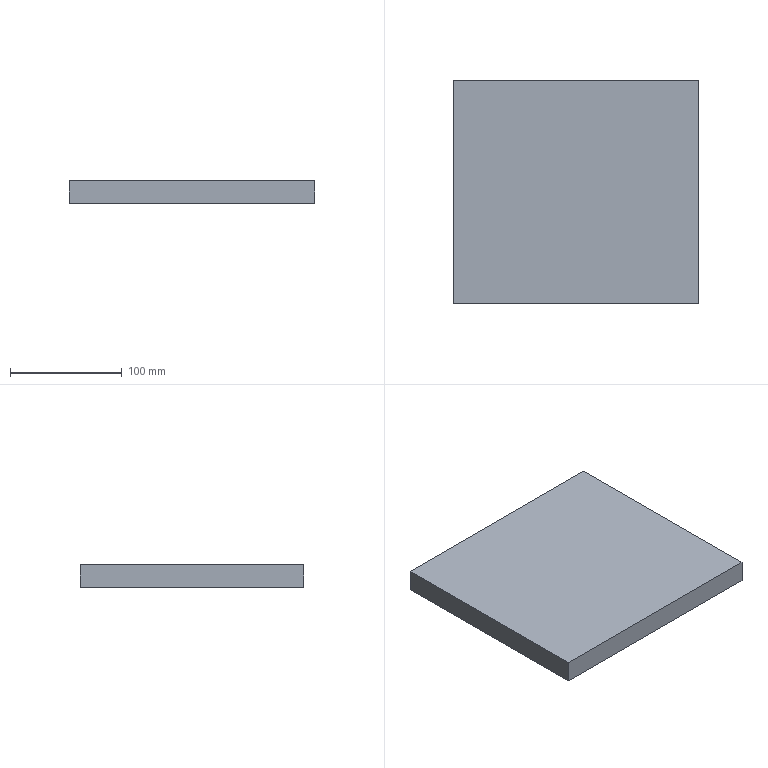Part | NX | features BREP 1 | 1 solid | 6 faces | box 220 x 200 x 20 mm | volume 880000 mm3 | plane 6
STEP:
#1=CARTESIAN_POINT('',(-110.,100.,-10.));
#2=VERTEX_POINT('',#1);
#3=CARTESIAN_POINT('',(-110.,-100.,-10.));
#4=VERTEX_POINT('',#3);
#5=CARTESIAN_POINT('',(-110.,100.,-10.));
#6=DIRECTION('',(0.,-1.,0.));
#7=VECTOR('',#6,1000.);
#8=LINE('',#5,#7);
#9=EDGE_CURVE('',#2,#4,#8,.T.);
#10=ORIENTED_EDGE('',*,*,#9,.T.);
#11=CARTESIAN_POINT('',(-110.,-100.,10.));
#12=VERTEX_POINT('',#11);
#13=CARTESIAN_POINT('',(-110.,-100.,10.));
#14=DIRECTION('',(0.,0.,-1.));
#15=VECTOR('',#14,1000.);
#16=LINE('',#13,#15);
#17=EDGE_CURVE('',#12,#4,#16,.T.);
#18=ORIENTED_EDGE('',*,*,#17,.F.);
#19=CARTESIAN_POINT('',(-110.,100.,10.));
#20=VERTEX_POINT('',#19);
#21=CARTESIAN_POINT('',(-110.,100.,10.));
#22=DIRECTION('',(0.,-1.,0.));
#23=VECTOR('',#22,1000.);
#24=LINE('',#21,#23);
#25=EDGE_CURVE('',#20,#12,#24,.T.);
#26=ORIENTED_EDGE('',*,*,#25,.F.);
#27=CARTESIAN_POINT('',(-110.,100.,10.));
#28=DIRECTION('',(0.,0.,-1.));
#29=VECTOR('',#28,1000.);
#30=LINE('',#27,#29);
#31=EDGE_CURVE('',#20,#2,#30,.T.);
#32=ORIENTED_EDGE('',*,*,#31,.T.);
#33=EDGE_LOOP('',(#10,#18,#26,#32));
#34=FACE_BOUND('',#33,.T.);
#35=CARTESIAN_POINT('',(-110.,100.,10.));
#36=DIRECTION('',(1.,0.,0.));
#37=DIRECTION('',(0.,0.,1.));
#38=AXIS2_PLACEMENT_3D('',#35,#36,#37);
#39=PLANE('',#38);
#40=ADVANCED_FACE('',(#34),#39,.F.);
#41=CARTESIAN_POINT('',(110.,-100.,-10.));
#42=VERTEX_POINT('',#41);
#43=CARTESIAN_POINT('',(-110.,-100.,-10.));
#44=DIRECTION('',(1.,0.,0.));
#45=VECTOR('',#44,1000.);
#46=LINE('',#43,#45);
#47=EDGE_CURVE('',#4,#42,#46,.T.);
#48=ORIENTED_EDGE('',*,*,#47,.T.);
#49=CARTESIAN_POINT('',(110.,-100.,10.));
#50=VERTEX_POINT('',#49);
#51=CARTESIAN_POINT('',(110.,-100.,10.));
#52=DIRECTION('',(0.,0.,-1.));
#53=VECTOR('',#52,1000.);
#54=LINE('',#51,#53);
#55=EDGE_CURVE('',#50,#42,#54,.T.);
#56=ORIENTED_EDGE('',*,*,#55,.F.);
#57=CARTESIAN_POINT('',(-110.,-100.,10.));
#58=DIRECTION('',(1.,0.,0.));
#59=VECTOR('',#58,1000.);
#60=LINE('',#57,#59);
#61=EDGE_CURVE('',#12,#50,#60,.T.);
#62=ORIENTED_EDGE('',*,*,#61,.F.);
#63=ORIENTED_EDGE('',*,*,#17,.T.);
#64=EDGE_LOOP('',(#48,#56,#62,#63));
#65=FACE_BOUND('',#64,.T.);
#66=CARTESIAN_POINT('',(-110.,-100.,10.));
#67=DIRECTION('',(0.,1.,0.));
#68=DIRECTION('',(0.,0.,-1.));
#69=AXIS2_PLACEMENT_3D('',#66,#67,#68);
#70=PLANE('',#69);
#71=ADVANCED_FACE('',(#65),#70,.F.);
#72=CARTESIAN_POINT('',(110.,100.,-10.));
#73=VERTEX_POINT('',#72);
#74=CARTESIAN_POINT('',(110.,100.,-10.));
#75=DIRECTION('',(0.,1.,0.));
#76=VECTOR('',#75,1000.);
#77=LINE('',#74,#76);
#78=EDGE_CURVE('',#42,#73,#77,.T.);
#79=ORIENTED_EDGE('',*,*,#78,.T.);
#80=CARTESIAN_POINT('',(110.,100.,10.));
#81=VERTEX_POINT('',#80);
#82=CARTESIAN_POINT('',(110.,100.,10.));
#83=DIRECTION('',(0.,0.,-1.));
#84=VECTOR('',#83,1000.);
#85=LINE('',#82,#84);
#86=EDGE_CURVE('',#81,#73,#85,.T.);
#87=ORIENTED_EDGE('',*,*,#86,.F.);
#88=CARTESIAN_POINT('',(110.,100.,10.));
#89=DIRECTION('',(0.,1.,0.));
#90=VECTOR('',#89,1000.);
#91=LINE('',#88,#90);
#92=EDGE_CURVE('',#50,#81,#91,.T.);
#93=ORIENTED_EDGE('',*,*,#92,.F.);
#94=ORIENTED_EDGE('',*,*,#55,.T.);
#95=EDGE_LOOP('',(#79,#87,#93,#94));
#96=FACE_BOUND('',#95,.T.);
#97=CARTESIAN_POINT('',(110.,100.,10.));
#98=DIRECTION('',(-1.,0.,0.));
#99=DIRECTION('',(0.,0.,-1.));
#100=AXIS2_PLACEMENT_3D('',#97,#98,#99);
#101=PLANE('',#100);
#102=ADVANCED_FACE('',(#96),#101,.F.);
#103=CARTESIAN_POINT('',(-110.,100.,-10.));
#104=DIRECTION('',(-1.,0.,0.));
#105=VECTOR('',#104,1000.);
#106=LINE('',#103,#105);
#107=EDGE_CURVE('',#73,#2,#106,.T.);
#108=ORIENTED_EDGE('',*,*,#107,.T.);
#109=ORIENTED_EDGE('',*,*,#31,.F.);
#110=CARTESIAN_POINT('',(-110.,100.,10.));
#111=DIRECTION('',(-1.,0.,0.));
#112=VECTOR('',#111,1000.);
#113=LINE('',#110,#112);
#114=EDGE_CURVE('',#81,#20,#113,.T.);
#115=ORIENTED_EDGE('',*,*,#114,.F.);
#116=ORIENTED_EDGE('',*,*,#86,.T.);
#117=EDGE_LOOP('',(#108,#109,#115,#116));
#118=FACE_BOUND('',#117,.T.);
#119=CARTESIAN_POINT('',(-110.,100.,10.));
#120=DIRECTION('',(0.,-1.,0.));
#121=DIRECTION('',(0.,0.,1.));
#122=AXIS2_PLACEMENT_3D('',#119,#120,#121);
#123=PLANE('',#122);
#124=ADVANCED_FACE('',(#118),#123,.F.);
#125=ORIENTED_EDGE('',*,*,#25,.T.);
#126=ORIENTED_EDGE('',*,*,#61,.T.);
#127=ORIENTED_EDGE('',*,*,#92,.T.);
#128=ORIENTED_EDGE('',*,*,#114,.T.);
#129=EDGE_LOOP('',(#125,#126,#127,#128));
#130=FACE_BOUND('',#129,.T.);
#131=CARTESIAN_POINT('',(-110.,-100.,10.));
#132=DIRECTION('',(0.,0.,1.));
#133=DIRECTION('',(-1.,0.,0.));
#134=AXIS2_PLACEMENT_3D('',#131,#132,#133);
#135=PLANE('',#134);
#136=ADVANCED_FACE('',(#130),#135,.T.);
#137=ORIENTED_EDGE('',*,*,#9,.F.);
#138=ORIENTED_EDGE('',*,*,#107,.F.);
#139=ORIENTED_EDGE('',*,*,#78,.F.);
#140=ORIENTED_EDGE('',*,*,#47,.F.);
#141=EDGE_LOOP('',(#137,#138,#139,#140));
#142=FACE_BOUND('',#141,.T.);
#143=CARTESIAN_POINT('',(-110.,-100.,-10.));
#144=DIRECTION('',(0.,0.,1.));
#145=DIRECTION('',(-1.,0.,0.));
#146=AXIS2_PLACEMENT_3D('',#143,#144,#145);
#147=PLANE('',#146);
#148=ADVANCED_FACE('',(#142),#147,.F.);
#149=CLOSED_SHELL('',(#40,#71,#102,#124,#136,#148));
#150=MANIFOLD_SOLID_BREP('',#149);
#151=(LENGTH_UNIT()NAMED_UNIT(*)SI_UNIT(.MILLI.,.METRE.));
#152=UNCERTAINTY_MEASURE_WITH_UNIT(LENGTH_MEASURE(0.00001),#151,'','');
#153=(NAMED_UNIT(*)PLANE_ANGLE_UNIT()SI_UNIT($,.RADIAN.));
#154=(NAMED_UNIT(*)SI_UNIT($,.STERADIAN.)SOLID_ANGLE_UNIT());
#155=(GEOMETRIC_REPRESENTATION_CONTEXT(3)GLOBAL_UNCERTAINTY_ASSIGNED_CONTEXT((#152))GLOBAL_UNIT_ASSIGNED_CONTEXT((#151,#153,#154))REPRESENTATION_CONTEXT('',''));
#156=ADVANCED_BREP_SHAPE_REPRESENTATION('',(#150),#155);